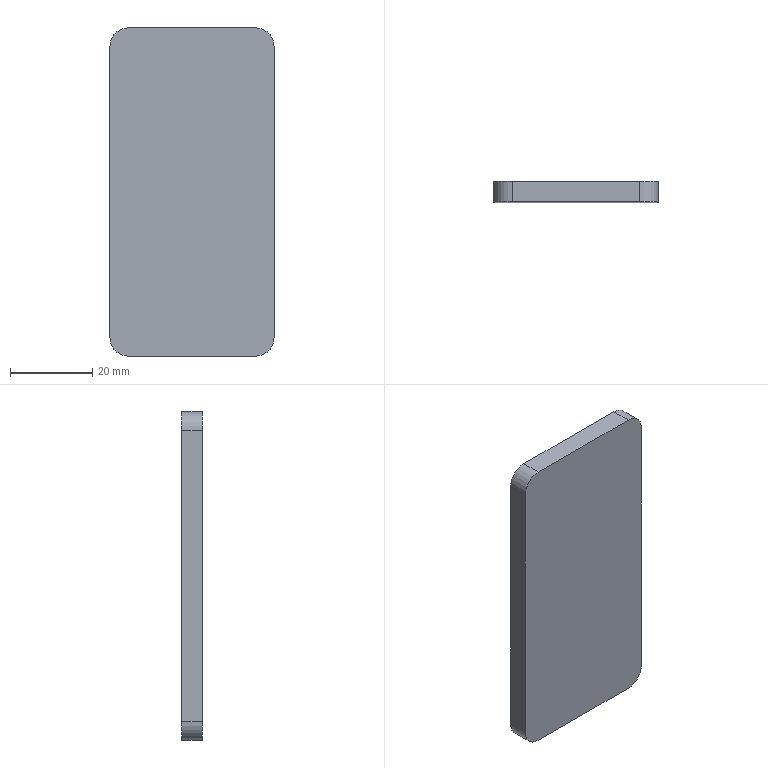Part | SolidWorks | features Extrusion 1, Fillet 1 | 1 solid | 10 faces | box 40 x 5 x 80 mm | volume 15913 mm3 | plane 6 | cylinder 4 | commonest cylinder face diameters 9 x4
STEP:
#1=CARTESIAN_POINT('',(20.,-2.5,35.5));
#2=VERTEX_POINT('',#1);
#3=CARTESIAN_POINT('',(20.,-2.5,-35.5));
#4=VERTEX_POINT('',#3);
#5=CARTESIAN_POINT('',(20.,-2.5,40.));
#6=DIRECTION('',(0.,0.,-1.));
#7=VECTOR('',#6,1000.);
#8=LINE('',#5,#7);
#9=EDGE_CURVE('',#2,#4,#8,.T.);
#10=ORIENTED_EDGE('',*,*,#9,.T.);
#11=CARTESIAN_POINT('',(20.,2.5,-35.5));
#12=VERTEX_POINT('',#11);
#13=CARTESIAN_POINT('',(20.,2.5,-35.5));
#14=DIRECTION('',(0.,1.,0.));
#15=VECTOR('',#14,1000.);
#16=LINE('',#13,#15);
#17=EDGE_CURVE('',#4,#12,#16,.T.);
#18=ORIENTED_EDGE('',*,*,#17,.T.);
#19=CARTESIAN_POINT('',(20.,2.5,35.5));
#20=VERTEX_POINT('',#19);
#21=CARTESIAN_POINT('',(20.,2.5,40.));
#22=DIRECTION('',(0.,0.,-1.));
#23=VECTOR('',#22,1000.);
#24=LINE('',#21,#23);
#25=EDGE_CURVE('',#20,#12,#24,.T.);
#26=ORIENTED_EDGE('',*,*,#25,.F.);
#27=CARTESIAN_POINT('',(20.,2.5,35.5));
#28=DIRECTION('',(0.,-1.,0.));
#29=VECTOR('',#28,1000.);
#30=LINE('',#27,#29);
#31=EDGE_CURVE('',#20,#2,#30,.T.);
#32=ORIENTED_EDGE('',*,*,#31,.T.);
#33=EDGE_LOOP('',(#10,#18,#26,#32));
#34=FACE_OUTER_BOUND('',#33,.T.);
#35=CARTESIAN_POINT('',(20.,2.5,40.));
#36=DIRECTION('',(-1.,0.,0.));
#37=DIRECTION('',(0.,0.,1.));
#38=AXIS2_PLACEMENT_3D('',#35,#36,#37);
#39=PLANE('',#38);
#40=ADVANCED_FACE('',(#34),#39,.F.);
#41=CARTESIAN_POINT('',(15.5,2.5,-40.));
#42=VERTEX_POINT('',#41);
#43=CARTESIAN_POINT('',(-15.5,2.5,-40.));
#44=VERTEX_POINT('',#43);
#45=CARTESIAN_POINT('',(-20.,2.5,-40.));
#46=DIRECTION('',(-1.,0.,0.));
#47=VECTOR('',#46,1000.);
#48=LINE('',#45,#47);
#49=EDGE_CURVE('',#42,#44,#48,.T.);
#50=ORIENTED_EDGE('',*,*,#49,.F.);
#51=CARTESIAN_POINT('',(15.5,-2.5,-40.));
#52=VERTEX_POINT('',#51);
#53=CARTESIAN_POINT('',(15.5,2.5,-40.));
#54=DIRECTION('',(0.,-1.,0.));
#55=VECTOR('',#54,1000.);
#56=LINE('',#53,#55);
#57=EDGE_CURVE('',#42,#52,#56,.T.);
#58=ORIENTED_EDGE('',*,*,#57,.T.);
#59=CARTESIAN_POINT('',(-15.5,-2.5,-40.));
#60=VERTEX_POINT('',#59);
#61=CARTESIAN_POINT('',(-20.,-2.5,-40.));
#62=DIRECTION('',(-1.,0.,0.));
#63=VECTOR('',#62,1000.);
#64=LINE('',#61,#63);
#65=EDGE_CURVE('',#52,#60,#64,.T.);
#66=ORIENTED_EDGE('',*,*,#65,.T.);
#67=CARTESIAN_POINT('',(-15.5,2.5,-40.));
#68=DIRECTION('',(0.,1.,0.));
#69=VECTOR('',#68,1000.);
#70=LINE('',#67,#69);
#71=EDGE_CURVE('',#60,#44,#70,.T.);
#72=ORIENTED_EDGE('',*,*,#71,.T.);
#73=EDGE_LOOP('',(#50,#58,#66,#72));
#74=FACE_OUTER_BOUND('',#73,.T.);
#75=CARTESIAN_POINT('',(-20.,2.5,-40.));
#76=DIRECTION('',(0.,0.,1.));
#77=DIRECTION('',(1.,0.,0.));
#78=AXIS2_PLACEMENT_3D('',#75,#76,#77);
#79=PLANE('',#78);
#80=ADVANCED_FACE('',(#74),#79,.F.);
#81=CARTESIAN_POINT('',(-20.,2.5,-35.5));
#82=VERTEX_POINT('',#81);
#83=CARTESIAN_POINT('',(-20.,2.5,35.5));
#84=VERTEX_POINT('',#83);
#85=CARTESIAN_POINT('',(-20.,2.5,40.));
#86=DIRECTION('',(0.,0.,1.));
#87=VECTOR('',#86,1000.);
#88=LINE('',#85,#87);
#89=EDGE_CURVE('',#82,#84,#88,.T.);
#90=ORIENTED_EDGE('',*,*,#89,.F.);
#91=CARTESIAN_POINT('',(-20.,-2.5,-35.5));
#92=VERTEX_POINT('',#91);
#93=CARTESIAN_POINT('',(-20.,2.5,-35.5));
#94=DIRECTION('',(0.,-1.,0.));
#95=VECTOR('',#94,1000.);
#96=LINE('',#93,#95);
#97=EDGE_CURVE('',#82,#92,#96,.T.);
#98=ORIENTED_EDGE('',*,*,#97,.T.);
#99=CARTESIAN_POINT('',(-20.,-2.5,35.5));
#100=VERTEX_POINT('',#99);
#101=CARTESIAN_POINT('',(-20.,-2.5,40.));
#102=DIRECTION('',(0.,0.,1.));
#103=VECTOR('',#102,1000.);
#104=LINE('',#101,#103);
#105=EDGE_CURVE('',#92,#100,#104,.T.);
#106=ORIENTED_EDGE('',*,*,#105,.T.);
#107=CARTESIAN_POINT('',(-20.,2.5,35.5));
#108=DIRECTION('',(0.,1.,0.));
#109=VECTOR('',#108,1000.);
#110=LINE('',#107,#109);
#111=EDGE_CURVE('',#100,#84,#110,.T.);
#112=ORIENTED_EDGE('',*,*,#111,.T.);
#113=EDGE_LOOP('',(#90,#98,#106,#112));
#114=FACE_OUTER_BOUND('',#113,.T.);
#115=CARTESIAN_POINT('',(-20.,2.5,40.));
#116=DIRECTION('',(1.,0.,0.));
#117=DIRECTION('',(0.,0.,-1.));
#118=AXIS2_PLACEMENT_3D('',#115,#116,#117);
#119=PLANE('',#118);
#120=ADVANCED_FACE('',(#114),#119,.F.);
#121=CARTESIAN_POINT('',(-15.5,-2.5,40.));
#122=VERTEX_POINT('',#121);
#123=CARTESIAN_POINT('',(15.5,-2.5,40.));
#124=VERTEX_POINT('',#123);
#125=CARTESIAN_POINT('',(-20.,-2.5,40.));
#126=DIRECTION('',(1.,0.,0.));
#127=VECTOR('',#126,1000.);
#128=LINE('',#125,#127);
#129=EDGE_CURVE('',#122,#124,#128,.T.);
#130=ORIENTED_EDGE('',*,*,#129,.T.);
#131=CARTESIAN_POINT('',(15.5,2.5,40.));
#132=VERTEX_POINT('',#131);
#133=CARTESIAN_POINT('',(15.5,2.5,40.));
#134=DIRECTION('',(0.,1.,0.));
#135=VECTOR('',#134,1000.);
#136=LINE('',#133,#135);
#137=EDGE_CURVE('',#124,#132,#136,.T.);
#138=ORIENTED_EDGE('',*,*,#137,.T.);
#139=CARTESIAN_POINT('',(-15.5,2.5,40.));
#140=VERTEX_POINT('',#139);
#141=CARTESIAN_POINT('',(-20.,2.5,40.));
#142=DIRECTION('',(1.,0.,0.));
#143=VECTOR('',#142,1000.);
#144=LINE('',#141,#143);
#145=EDGE_CURVE('',#140,#132,#144,.T.);
#146=ORIENTED_EDGE('',*,*,#145,.F.);
#147=CARTESIAN_POINT('',(-15.5,2.5,40.));
#148=DIRECTION('',(0.,-1.,0.));
#149=VECTOR('',#148,1000.);
#150=LINE('',#147,#149);
#151=EDGE_CURVE('',#140,#122,#150,.T.);
#152=ORIENTED_EDGE('',*,*,#151,.T.);
#153=EDGE_LOOP('',(#130,#138,#146,#152));
#154=FACE_OUTER_BOUND('',#153,.T.);
#155=CARTESIAN_POINT('',(-20.,2.5,40.));
#156=DIRECTION('',(0.,0.,-1.));
#157=DIRECTION('',(-1.,0.,0.));
#158=AXIS2_PLACEMENT_3D('',#155,#156,#157);
#159=PLANE('',#158);
#160=ADVANCED_FACE('',(#154),#159,.F.);
#161=ORIENTED_EDGE('',*,*,#25,.T.);
#162=CARTESIAN_POINT('',(15.5,2.5,-35.5));
#163=DIRECTION('',(0.,1.,0.));
#164=DIRECTION('',(0.,0.,-1.));
#165=AXIS2_PLACEMENT_3D('',#162,#163,#164);
#166=CIRCLE('',#165,4.5);
#167=EDGE_CURVE('',#12,#42,#166,.T.);
#168=ORIENTED_EDGE('',*,*,#167,.T.);
#169=ORIENTED_EDGE('',*,*,#49,.T.);
#170=CARTESIAN_POINT('',(-15.5,2.5,-35.5));
#171=DIRECTION('',(0.,1.,0.));
#172=DIRECTION('',(0.,0.,-1.));
#173=AXIS2_PLACEMENT_3D('',#170,#171,#172);
#174=CIRCLE('',#173,4.5);
#175=EDGE_CURVE('',#44,#82,#174,.T.);
#176=ORIENTED_EDGE('',*,*,#175,.T.);
#177=ORIENTED_EDGE('',*,*,#89,.T.);
#178=CARTESIAN_POINT('',(-15.5,2.5,35.5));
#179=DIRECTION('',(0.,1.,0.));
#180=DIRECTION('',(0.,0.,-1.));
#181=AXIS2_PLACEMENT_3D('',#178,#179,#180);
#182=CIRCLE('',#181,4.5);
#183=EDGE_CURVE('',#84,#140,#182,.T.);
#184=ORIENTED_EDGE('',*,*,#183,.T.);
#185=ORIENTED_EDGE('',*,*,#145,.T.);
#186=CARTESIAN_POINT('',(15.5,2.5,35.5));
#187=DIRECTION('',(0.,1.,0.));
#188=DIRECTION('',(0.,0.,-1.));
#189=AXIS2_PLACEMENT_3D('',#186,#187,#188);
#190=CIRCLE('',#189,4.5);
#191=EDGE_CURVE('',#132,#20,#190,.T.);
#192=ORIENTED_EDGE('',*,*,#191,.T.);
#193=EDGE_LOOP('',(#161,#168,#169,#176,#177,#184,#185,#192));
#194=FACE_OUTER_BOUND('',#193,.T.);
#195=CARTESIAN_POINT('',(0.,2.5,0.));
#196=DIRECTION('',(0.,-1.,0.));
#197=DIRECTION('',(0.,0.,-1.));
#198=AXIS2_PLACEMENT_3D('',#195,#196,#197);
#199=PLANE('',#198);
#200=ADVANCED_FACE('',(#194),#199,.F.);
#201=ORIENTED_EDGE('',*,*,#65,.F.);
#202=CARTESIAN_POINT('',(15.5,-2.5,-35.5));
#203=DIRECTION('',(0.,-1.,0.));
#204=DIRECTION('',(0.,0.,-1.));
#205=AXIS2_PLACEMENT_3D('',#202,#203,#204);
#206=CIRCLE('',#205,4.5);
#207=EDGE_CURVE('',#52,#4,#206,.T.);
#208=ORIENTED_EDGE('',*,*,#207,.T.);
#209=ORIENTED_EDGE('',*,*,#9,.F.);
#210=CARTESIAN_POINT('',(15.5,-2.5,35.5));
#211=DIRECTION('',(0.,-1.,0.));
#212=DIRECTION('',(0.,0.,-1.));
#213=AXIS2_PLACEMENT_3D('',#210,#211,#212);
#214=CIRCLE('',#213,4.5);
#215=EDGE_CURVE('',#2,#124,#214,.T.);
#216=ORIENTED_EDGE('',*,*,#215,.T.);
#217=ORIENTED_EDGE('',*,*,#129,.F.);
#218=CARTESIAN_POINT('',(-15.5,-2.5,35.5));
#219=DIRECTION('',(0.,-1.,0.));
#220=DIRECTION('',(0.,0.,-1.));
#221=AXIS2_PLACEMENT_3D('',#218,#219,#220);
#222=CIRCLE('',#221,4.5);
#223=EDGE_CURVE('',#122,#100,#222,.T.);
#224=ORIENTED_EDGE('',*,*,#223,.T.);
#225=ORIENTED_EDGE('',*,*,#105,.F.);
#226=CARTESIAN_POINT('',(-15.5,-2.5,-35.5));
#227=DIRECTION('',(0.,-1.,0.));
#228=DIRECTION('',(0.,0.,-1.));
#229=AXIS2_PLACEMENT_3D('',#226,#227,#228);
#230=CIRCLE('',#229,4.5);
#231=EDGE_CURVE('',#92,#60,#230,.T.);
#232=ORIENTED_EDGE('',*,*,#231,.T.);
#233=EDGE_LOOP('',(#201,#208,#209,#216,#217,#224,#225,#232));
#234=FACE_OUTER_BOUND('',#233,.T.);
#235=CARTESIAN_POINT('',(0.,-2.5,0.));
#236=DIRECTION('',(0.,-1.,0.));
#237=DIRECTION('',(0.,0.,-1.));
#238=AXIS2_PLACEMENT_3D('',#235,#236,#237);
#239=PLANE('',#238);
#240=ADVANCED_FACE('',(#234),#239,.T.);
#241=ORIENTED_EDGE('',*,*,#167,.F.);
#242=ORIENTED_EDGE('',*,*,#17,.F.);
#243=ORIENTED_EDGE('',*,*,#207,.F.);
#244=ORIENTED_EDGE('',*,*,#57,.F.);
#245=EDGE_LOOP('',(#241,#242,#243,#244));
#246=FACE_OUTER_BOUND('',#245,.T.);
#247=CARTESIAN_POINT('',(15.5,2.5,-35.5));
#248=DIRECTION('',(0.,-1.,0.));
#249=DIRECTION('',(0.,0.,-1.));
#250=AXIS2_PLACEMENT_3D('',#247,#248,#249);
#251=CYLINDRICAL_SURFACE('',#250,4.5);
#252=ADVANCED_FACE('',(#246),#251,.T.);
#253=ORIENTED_EDGE('',*,*,#191,.F.);
#254=ORIENTED_EDGE('',*,*,#137,.F.);
#255=ORIENTED_EDGE('',*,*,#215,.F.);
#256=ORIENTED_EDGE('',*,*,#31,.F.);
#257=EDGE_LOOP('',(#253,#254,#255,#256));
#258=FACE_OUTER_BOUND('',#257,.T.);
#259=CARTESIAN_POINT('',(15.5,2.5,35.5));
#260=DIRECTION('',(0.,-1.,0.));
#261=DIRECTION('',(0.,0.,-1.));
#262=AXIS2_PLACEMENT_3D('',#259,#260,#261);
#263=CYLINDRICAL_SURFACE('',#262,4.5);
#264=ADVANCED_FACE('',(#258),#263,.T.);
#265=ORIENTED_EDGE('',*,*,#175,.F.);
#266=ORIENTED_EDGE('',*,*,#71,.F.);
#267=ORIENTED_EDGE('',*,*,#231,.F.);
#268=ORIENTED_EDGE('',*,*,#97,.F.);
#269=EDGE_LOOP('',(#265,#266,#267,#268));
#270=FACE_OUTER_BOUND('',#269,.T.);
#271=CARTESIAN_POINT('',(-15.5,2.5,-35.5));
#272=DIRECTION('',(0.,-1.,0.));
#273=DIRECTION('',(0.,0.,-1.));
#274=AXIS2_PLACEMENT_3D('',#271,#272,#273);
#275=CYLINDRICAL_SURFACE('',#274,4.5);
#276=ADVANCED_FACE('',(#270),#275,.T.);
#277=ORIENTED_EDGE('',*,*,#183,.F.);
#278=ORIENTED_EDGE('',*,*,#111,.F.);
#279=ORIENTED_EDGE('',*,*,#223,.F.);
#280=ORIENTED_EDGE('',*,*,#151,.F.);
#281=EDGE_LOOP('',(#277,#278,#279,#280));
#282=FACE_OUTER_BOUND('',#281,.T.);
#283=CARTESIAN_POINT('',(-15.5,2.5,35.5));
#284=DIRECTION('',(0.,-1.,0.));
#285=DIRECTION('',(0.,0.,-1.));
#286=AXIS2_PLACEMENT_3D('',#283,#284,#285);
#287=CYLINDRICAL_SURFACE('',#286,4.5);
#288=ADVANCED_FACE('',(#282),#287,.T.);
#289=CLOSED_SHELL('',(#40,#80,#120,#160,#200,#240,#252,#264,#276,#288));
#290=MANIFOLD_SOLID_BREP('',#289);
#291=CARTESIAN_POINT('',(0.,0.,0.));
#292=DIRECTION('',(0.,0.,1.));
#293=DIRECTION('',(1.,0.,0.));
#294=AXIS2_PLACEMENT_3D('',#291,#292,#293);
#295=(LENGTH_UNIT()NAMED_UNIT(*)SI_UNIT(.MILLI.,.METRE.));
#296=UNCERTAINTY_MEASURE_WITH_UNIT(LENGTH_MEASURE(0.00001),#295,'','');
#297=(NAMED_UNIT(*)PLANE_ANGLE_UNIT()SI_UNIT($,.RADIAN.));
#298=(NAMED_UNIT(*)SI_UNIT($,.STERADIAN.)SOLID_ANGLE_UNIT());
#299=(GEOMETRIC_REPRESENTATION_CONTEXT(3)GLOBAL_UNCERTAINTY_ASSIGNED_CONTEXT((#296))GLOBAL_UNIT_ASSIGNED_CONTEXT((#295,#297,#298))REPRESENTATION_CONTEXT('',''));
#300=ADVANCED_BREP_SHAPE_REPRESENTATION('',(#290,#294),#299);